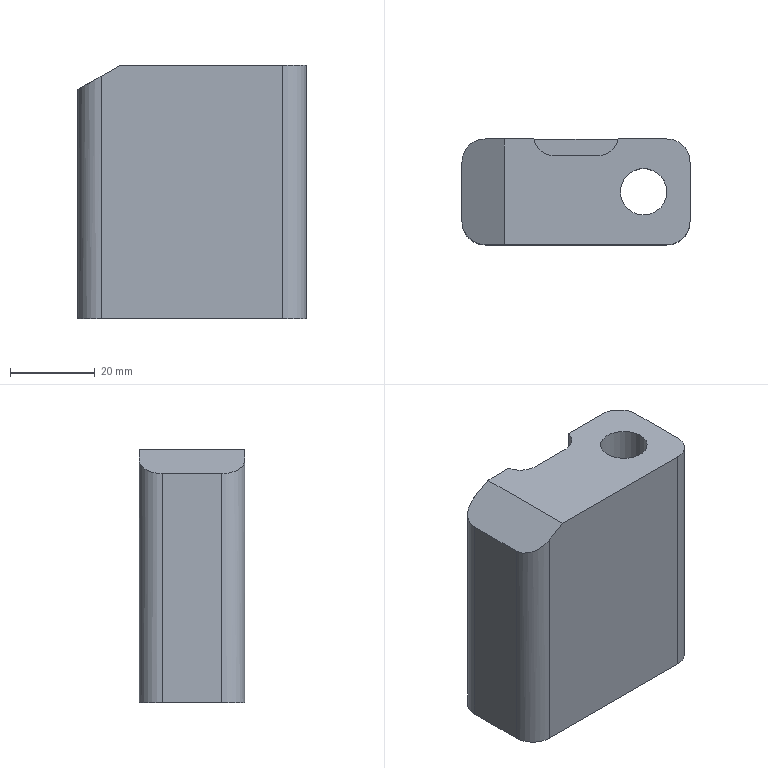Part | NX | features 1605338300 2 | 1 solid | 20 faces | box 54 x 25 x 60 mm | volume 60938 mm3 | plane 11 | cylinder 9 | commonest cylinder face diameters 11 x5 10 x2 17 x2
STEP:
#1=CARTESIAN_POINT('',(149.5,0.000000002,-61.5));
#2=VERTEX_POINT('',#1);
#3=CARTESIAN_POINT('',(158.,0.000000002,-61.5));
#4=DIRECTION('',(0.,0.,-1.));
#5=DIRECTION('',(-1.,0.,0.));
#6=AXIS2_PLACEMENT_3D('',#3,#4,#5);
#7=CIRCLE('',#6,8.5);
#8=EDGE_CURVE('',#2,#2,#7,.F.);
#9=ORIENTED_EDGE('',*,*,#8,.T.);
#10=EDGE_LOOP('',(#9));
#11=FACE_BOUND('',#10,.T.);
#12=CARTESIAN_POINT('',(147.,-7.,-61.5));
#13=VERTEX_POINT('',#12);
#14=CARTESIAN_POINT('',(147.,7.,-61.5));
#15=VERTEX_POINT('',#14);
#16=CARTESIAN_POINT('',(147.,-5.,-61.5));
#17=DIRECTION('',(0.,1.,0.));
#18=VECTOR('',#17,1000.);
#19=LINE('',#16,#18);
#20=EDGE_CURVE('',#13,#15,#19,.T.);
#21=ORIENTED_EDGE('',*,*,#20,.T.);
#22=CARTESIAN_POINT('',(152.5,12.5,-61.5));
#23=VERTEX_POINT('',#22);
#24=CARTESIAN_POINT('',(152.5,7.,-61.5));
#25=DIRECTION('',(0.,0.,-1.));
#26=DIRECTION('',(-1.,0.,0.));
#27=AXIS2_PLACEMENT_3D('',#24,#25,#26);
#28=CIRCLE('',#27,5.5);
#29=EDGE_CURVE('',#23,#15,#28,.F.);
#30=ORIENTED_EDGE('',*,*,#29,.F.);
#31=CARTESIAN_POINT('',(195.5,12.5,-61.5));
#32=VERTEX_POINT('',#31);
#33=CARTESIAN_POINT('',(159.,12.5,-61.5));
#34=DIRECTION('',(1.,0.,0.));
#35=VECTOR('',#34,1000.);
#36=LINE('',#33,#35);
#37=EDGE_CURVE('',#23,#32,#36,.T.);
#38=ORIENTED_EDGE('',*,*,#37,.T.);
#39=CARTESIAN_POINT('',(201.,7.,-61.5));
#40=VERTEX_POINT('',#39);
#41=CARTESIAN_POINT('',(195.5,7.,-61.5));
#42=DIRECTION('',(0.,0.,-1.));
#43=DIRECTION('',(-1.,0.,0.));
#44=AXIS2_PLACEMENT_3D('',#41,#42,#43);
#45=CIRCLE('',#44,5.5);
#46=EDGE_CURVE('',#40,#32,#45,.F.);
#47=ORIENTED_EDGE('',*,*,#46,.F.);
#48=CARTESIAN_POINT('',(201.,-7.,-61.5));
#49=VERTEX_POINT('',#48);
#50=CARTESIAN_POINT('',(201.,-5.,-61.5));
#51=DIRECTION('',(0.,-1.,0.));
#52=VECTOR('',#51,1000.);
#53=LINE('',#50,#52);
#54=EDGE_CURVE('',#40,#49,#53,.T.);
#55=ORIENTED_EDGE('',*,*,#54,.T.);
#56=CARTESIAN_POINT('',(195.5,-12.5,-61.5));
#57=VERTEX_POINT('',#56);
#58=CARTESIAN_POINT('',(195.5,-7.,-61.5));
#59=DIRECTION('',(0.,0.,-1.));
#60=DIRECTION('',(-1.,0.,0.));
#61=AXIS2_PLACEMENT_3D('',#58,#59,#60);
#62=CIRCLE('',#61,5.5);
#63=EDGE_CURVE('',#57,#49,#62,.F.);
#64=ORIENTED_EDGE('',*,*,#63,.F.);
#65=CARTESIAN_POINT('',(152.5,-12.5,-61.5));
#66=VERTEX_POINT('',#65);
#67=CARTESIAN_POINT('',(159.,-12.5,-61.5));
#68=DIRECTION('',(-1.,0.,0.));
#69=VECTOR('',#68,1000.);
#70=LINE('',#67,#69);
#71=EDGE_CURVE('',#57,#66,#70,.T.);
#72=ORIENTED_EDGE('',*,*,#71,.T.);
#73=CARTESIAN_POINT('',(152.5,-7.,-61.5));
#74=DIRECTION('',(0.,0.,-1.));
#75=DIRECTION('',(-1.,0.,0.));
#76=AXIS2_PLACEMENT_3D('',#73,#74,#75);
#77=CIRCLE('',#76,5.5);
#78=EDGE_CURVE('',#13,#66,#77,.F.);
#79=ORIENTED_EDGE('',*,*,#78,.F.);
#80=EDGE_LOOP('',(#21,#30,#38,#47,#55,#64,#72,#79));
#81=FACE_BOUND('',#80,.T.);
#82=CARTESIAN_POINT('',(181.5,0.000000002,-61.5));
#83=VERTEX_POINT('',#82);
#84=CARTESIAN_POINT('',(190.,0.000000002,-61.5));
#85=DIRECTION('',(0.,0.,-1.));
#86=DIRECTION('',(-1.,0.,0.));
#87=AXIS2_PLACEMENT_3D('',#84,#85,#86);
#88=CIRCLE('',#87,8.5);
#89=EDGE_CURVE('',#83,#83,#88,.F.);
#90=ORIENTED_EDGE('',*,*,#89,.T.);
#91=EDGE_LOOP('',(#90));
#92=FACE_BOUND('',#91,.T.);
#93=CARTESIAN_POINT('',(159.,-5.,-61.5));
#94=DIRECTION('',(0.,0.,-1.));
#95=DIRECTION('',(-1.,0.,0.));
#96=AXIS2_PLACEMENT_3D('',#93,#94,#95);
#97=PLANE('',#96);
#98=ADVANCED_FACE('',(#11,#81,#92),#97,.T.);
#99=CARTESIAN_POINT('',(181.5,0.000000002,-34.5));
#100=VERTEX_POINT('',#99);
#101=CARTESIAN_POINT('',(190.,0.000000002,-34.5));
#102=DIRECTION('',(0.,0.,-1.));
#103=DIRECTION('',(-1.,0.,0.));
#104=AXIS2_PLACEMENT_3D('',#101,#102,#103);
#105=CIRCLE('',#104,8.5);
#106=EDGE_CURVE('',#100,#100,#105,.T.);
#107=ORIENTED_EDGE('',*,*,#106,.F.);
#108=EDGE_LOOP('',(#107));
#109=FACE_BOUND('',#108,.T.);
#110=ORIENTED_EDGE('',*,*,#89,.F.);
#111=EDGE_LOOP('',(#110));
#112=FACE_BOUND('',#111,.T.);
#113=CARTESIAN_POINT('',(190.,0.000000002,-34.5));
#114=DIRECTION('',(0.,0.,-1.));
#115=DIRECTION('',(-1.,0.,0.));
#116=AXIS2_PLACEMENT_3D('',#113,#114,#115);
#117=CYLINDRICAL_SURFACE('',#116,8.5);
#118=ADVANCED_FACE('',(#109,#112),#117,.F.);
#119=CARTESIAN_POINT('',(184.5,0.,-34.5));
#120=VERTEX_POINT('',#119);
#121=CARTESIAN_POINT('',(190.,0.,-34.5));
#122=DIRECTION('',(0.,0.,-1.));
#123=DIRECTION('',(-1.,0.,0.));
#124=AXIS2_PLACEMENT_3D('',#121,#122,#123);
#125=CIRCLE('',#124,5.5);
#126=EDGE_CURVE('',#120,#120,#125,.T.);
#127=ORIENTED_EDGE('',*,*,#126,.T.);
#128=EDGE_LOOP('',(#127));
#129=FACE_BOUND('',#128,.T.);
#130=CARTESIAN_POINT('',(195.5,0.,-1.5));
#131=VERTEX_POINT('',#130);
#132=CARTESIAN_POINT('',(190.,0.,-1.5));
#133=DIRECTION('',(0.,0.,1.));
#134=DIRECTION('',(1.,0.,0.));
#135=AXIS2_PLACEMENT_3D('',#132,#133,#134);
#136=CIRCLE('',#135,5.5);
#137=EDGE_CURVE('',#131,#131,#136,.F.);
#138=ORIENTED_EDGE('',*,*,#137,.F.);
#139=EDGE_LOOP('',(#138));
#140=FACE_BOUND('',#139,.T.);
#141=CARTESIAN_POINT('',(190.,0.,20.5));
#142=DIRECTION('',(0.,0.,-1.));
#143=DIRECTION('',(-1.,0.,0.));
#144=AXIS2_PLACEMENT_3D('',#141,#142,#143);
#145=CYLINDRICAL_SURFACE('',#144,5.5);
#146=ADVANCED_FACE('',(#129,#140),#145,.F.);
#147=ORIENTED_EDGE('',*,*,#137,.T.);
#148=EDGE_LOOP('',(#147));
#149=FACE_BOUND('',#148,.T.);
#150=CARTESIAN_POINT('',(168.899,8.5,-1.5));
#151=VERTEX_POINT('',#150);
#152=CARTESIAN_POINT('',(179.101,8.5,-1.5));
#153=VERTEX_POINT('',#152);
#154=CARTESIAN_POINT('',(170.,8.5,-1.5));
#155=DIRECTION('',(1.,0.,0.));
#156=VECTOR('',#155,1000.);
#157=LINE('',#154,#156);
#158=EDGE_CURVE('',#151,#153,#157,.T.);
#159=ORIENTED_EDGE('',*,*,#158,.F.);
#160=CARTESIAN_POINT('',(164.,12.5,-1.5));
#161=VERTEX_POINT('',#160);
#162=CARTESIAN_POINT('',(168.899,13.5,-1.5));
#163=DIRECTION('',(0.,0.,-1.));
#164=DIRECTION('',(1.,0.,0.));
#165=AXIS2_PLACEMENT_3D('',#162,#163,#164);
#166=CIRCLE('',#165,5.);
#167=EDGE_CURVE('',#161,#151,#166,.F.);
#168=ORIENTED_EDGE('',*,*,#167,.F.);
#169=CARTESIAN_POINT('',(157.,12.5,-1.5));
#170=VERTEX_POINT('',#169);
#171=CARTESIAN_POINT('',(159.,12.5,-1.5));
#172=DIRECTION('',(-1.,0.,0.));
#173=VECTOR('',#172,1000.);
#174=LINE('',#171,#173);
#175=EDGE_CURVE('',#161,#170,#174,.T.);
#176=ORIENTED_EDGE('',*,*,#175,.T.);
#177=CARTESIAN_POINT('',(157.,-12.5,-1.5));
#178=VERTEX_POINT('',#177);
#179=CARTESIAN_POINT('',(157.,-5.,-1.5));
#180=DIRECTION('',(0.,1.,0.));
#181=VECTOR('',#180,1000.);
#182=LINE('',#179,#181);
#183=EDGE_CURVE('',#178,#170,#182,.T.);
#184=ORIENTED_EDGE('',*,*,#183,.F.);
#185=CARTESIAN_POINT('',(195.5,-12.5,-1.5));
#186=VERTEX_POINT('',#185);
#187=CARTESIAN_POINT('',(159.,-12.5,-1.5));
#188=DIRECTION('',(1.,0.,0.));
#189=VECTOR('',#188,1000.);
#190=LINE('',#187,#189);
#191=EDGE_CURVE('',#178,#186,#190,.T.);
#192=ORIENTED_EDGE('',*,*,#191,.T.);
#193=CARTESIAN_POINT('',(201.,-7.,-1.5));
#194=VERTEX_POINT('',#193);
#195=CARTESIAN_POINT('',(195.5,-7.,-1.5));
#196=DIRECTION('',(0.,0.,1.));
#197=DIRECTION('',(1.,0.,0.));
#198=AXIS2_PLACEMENT_3D('',#195,#196,#197);
#199=CIRCLE('',#198,5.5);
#200=EDGE_CURVE('',#194,#186,#199,.F.);
#201=ORIENTED_EDGE('',*,*,#200,.F.);
#202=CARTESIAN_POINT('',(201.,7.,-1.5));
#203=VERTEX_POINT('',#202);
#204=CARTESIAN_POINT('',(201.,-5.,-1.5));
#205=DIRECTION('',(0.,1.,0.));
#206=VECTOR('',#205,1000.);
#207=LINE('',#204,#206);
#208=EDGE_CURVE('',#194,#203,#207,.T.);
#209=ORIENTED_EDGE('',*,*,#208,.T.);
#210=CARTESIAN_POINT('',(195.5,12.5,-1.5));
#211=VERTEX_POINT('',#210);
#212=CARTESIAN_POINT('',(195.5,7.,-1.5));
#213=DIRECTION('',(0.,0.,1.));
#214=DIRECTION('',(1.,0.,0.));
#215=AXIS2_PLACEMENT_3D('',#212,#213,#214);
#216=CIRCLE('',#215,5.5);
#217=EDGE_CURVE('',#211,#203,#216,.F.);
#218=ORIENTED_EDGE('',*,*,#217,.F.);
#219=CARTESIAN_POINT('',(184.,12.5,-1.5));
#220=VERTEX_POINT('',#219);
#221=CARTESIAN_POINT('',(159.,12.5,-1.5));
#222=DIRECTION('',(-1.,0.,0.));
#223=VECTOR('',#222,1000.);
#224=LINE('',#221,#223);
#225=EDGE_CURVE('',#211,#220,#224,.T.);
#226=ORIENTED_EDGE('',*,*,#225,.T.);
#227=CARTESIAN_POINT('',(179.101,13.5,-1.5));
#228=DIRECTION('',(0.,0.,-1.));
#229=DIRECTION('',(1.,0.,0.));
#230=AXIS2_PLACEMENT_3D('',#227,#228,#229);
#231=CIRCLE('',#230,5.);
#232=EDGE_CURVE('',#153,#220,#231,.F.);
#233=ORIENTED_EDGE('',*,*,#232,.F.);
#234=EDGE_LOOP('',(#159,#168,#176,#184,#192,#201,#209,#218,#226,#233));
#235=FACE_BOUND('',#234,.T.);
#236=CARTESIAN_POINT('',(159.,-5.,-1.5));
#237=DIRECTION('',(0.,0.,1.));
#238=DIRECTION('',(1.,0.,0.));
#239=AXIS2_PLACEMENT_3D('',#236,#237,#238);
#240=PLANE('',#239);
#241=ADVANCED_FACE('',(#149,#235),#240,.T.);
#242=ORIENTED_EDGE('',*,*,#71,.F.);
#243=CARTESIAN_POINT('',(195.5,-12.5,-1.5));
#244=DIRECTION('',(0.,0.,-1.));
#245=VECTOR('',#244,1000.);
#246=LINE('',#243,#245);
#247=EDGE_CURVE('',#186,#57,#246,.T.);
#248=ORIENTED_EDGE('',*,*,#247,.F.);
#249=ORIENTED_EDGE('',*,*,#191,.F.);
#250=CARTESIAN_POINT('',(152.5,-12.5,-4.098));
#251=VERTEX_POINT('',#250);
#252=CARTESIAN_POINT('',(157.,-12.5,-1.5));
#253=DIRECTION('',(-0.866,0.,-0.5));
#254=VECTOR('',#253,1000.);
#255=LINE('',#252,#254);
#256=EDGE_CURVE('',#251,#178,#255,.F.);
#257=ORIENTED_EDGE('',*,*,#256,.F.);
#258=CARTESIAN_POINT('',(152.5,-12.5,-1.5));
#259=DIRECTION('',(0.,0.,-1.));
#260=VECTOR('',#259,1000.);
#261=LINE('',#258,#260);
#262=EDGE_CURVE('',#66,#251,#261,.F.);
#263=ORIENTED_EDGE('',*,*,#262,.F.);
#264=EDGE_LOOP('',(#242,#248,#249,#257,#263));
#265=FACE_BOUND('',#264,.T.);
#266=CARTESIAN_POINT('',(159.,-12.5,-1.5));
#267=DIRECTION('',(0.,-1.,0.));
#268=DIRECTION('',(0.,0.,1.));
#269=AXIS2_PLACEMENT_3D('',#266,#267,#268);
#270=PLANE('',#269);
#271=ADVANCED_FACE('',(#265),#270,.T.);
#272=CARTESIAN_POINT('',(147.,7.,-7.274));
#273=VERTEX_POINT('',#272);
#274=CARTESIAN_POINT('',(147.,-7.,-7.274));
#275=VERTEX_POINT('',#274);
#276=CARTESIAN_POINT('',(147.,-5.,-7.274));
#277=DIRECTION('',(0.,-1.,0.));
#278=VECTOR('',#277,1000.);
#279=LINE('',#276,#278);
#280=EDGE_CURVE('',#273,#275,#279,.T.);
#281=ORIENTED_EDGE('',*,*,#280,.F.);
#282=CARTESIAN_POINT('',(147.,7.,-1.5));
#283=DIRECTION('',(0.,0.,-1.));
#284=VECTOR('',#283,1000.);
#285=LINE('',#282,#284);
#286=EDGE_CURVE('',#15,#273,#285,.F.);
#287=ORIENTED_EDGE('',*,*,#286,.F.);
#288=ORIENTED_EDGE('',*,*,#20,.F.);
#289=CARTESIAN_POINT('',(147.,-7.,-1.5));
#290=DIRECTION('',(0.,0.,-1.));
#291=VECTOR('',#290,1000.);
#292=LINE('',#289,#291);
#293=EDGE_CURVE('',#275,#13,#292,.T.);
#294=ORIENTED_EDGE('',*,*,#293,.F.);
#295=EDGE_LOOP('',(#281,#287,#288,#294));
#296=FACE_BOUND('',#295,.T.);
#297=CARTESIAN_POINT('',(147.,-5.,-1.5));
#298=DIRECTION('',(-1.,0.,0.));
#299=DIRECTION('',(0.,0.,1.));
#300=AXIS2_PLACEMENT_3D('',#297,#298,#299);
#301=PLANE('',#300);
#302=ADVANCED_FACE('',(#296),#301,.T.);
#303=CARTESIAN_POINT('',(164.,12.5,-36.5));
#304=VERTEX_POINT('',#303);
#305=CARTESIAN_POINT('',(164.,12.5,-1.5));
#306=DIRECTION('',(0.,0.,-1.));
#307=VECTOR('',#306,1000.);
#308=LINE('',#305,#307);
#309=EDGE_CURVE('',#161,#304,#308,.T.);
#310=ORIENTED_EDGE('',*,*,#309,.T.);
#311=CARTESIAN_POINT('',(184.,12.5,-36.5));
#312=VERTEX_POINT('',#311);
#313=CARTESIAN_POINT('',(159.,12.5,-36.5));
#314=DIRECTION('',(1.,0.,0.));
#315=VECTOR('',#314,1000.);
#316=LINE('',#313,#315);
#317=EDGE_CURVE('',#304,#312,#316,.T.);
#318=ORIENTED_EDGE('',*,*,#317,.T.);
#319=CARTESIAN_POINT('',(184.,12.5,-1.5));
#320=DIRECTION('',(0.,0.,1.));
#321=VECTOR('',#320,1000.);
#322=LINE('',#319,#321);
#323=EDGE_CURVE('',#312,#220,#322,.T.);
#324=ORIENTED_EDGE('',*,*,#323,.T.);
#325=ORIENTED_EDGE('',*,*,#225,.F.);
#326=CARTESIAN_POINT('',(195.5,12.5,-1.5));
#327=DIRECTION('',(0.,0.,-1.));
#328=VECTOR('',#327,1000.);
#329=LINE('',#326,#328);
#330=EDGE_CURVE('',#32,#211,#329,.F.);
#331=ORIENTED_EDGE('',*,*,#330,.F.);
#332=ORIENTED_EDGE('',*,*,#37,.F.);
#333=CARTESIAN_POINT('',(152.5,12.5,-4.098));
#334=VERTEX_POINT('',#333);
#335=CARTESIAN_POINT('',(152.5,12.5,-1.5));
#336=DIRECTION('',(0.,0.,-1.));
#337=VECTOR('',#336,1000.);
#338=LINE('',#335,#337);
#339=EDGE_CURVE('',#334,#23,#338,.T.);
#340=ORIENTED_EDGE('',*,*,#339,.F.);
#341=CARTESIAN_POINT('',(157.,12.5,-1.5));
#342=DIRECTION('',(0.866,0.,0.5));
#343=VECTOR('',#342,1000.);
#344=LINE('',#341,#343);
#345=EDGE_CURVE('',#170,#334,#344,.F.);
#346=ORIENTED_EDGE('',*,*,#345,.F.);
#347=ORIENTED_EDGE('',*,*,#175,.F.);
#348=EDGE_LOOP('',(#310,#318,#324,#325,#331,#332,#340,#346,#347));
#349=FACE_BOUND('',#348,.T.);
#350=CARTESIAN_POINT('',(159.,12.5,-1.5));
#351=DIRECTION('',(0.,1.,0.));
#352=DIRECTION('',(0.,0.,-1.));
#353=AXIS2_PLACEMENT_3D('',#350,#351,#352);
#354=PLANE('',#353);
#355=ADVANCED_FACE('',(#349),#354,.T.);
#356=ORIENTED_EDGE('',*,*,#54,.F.);
#357=CARTESIAN_POINT('',(201.,7.,-1.5));
#358=DIRECTION('',(0.,0.,-1.));
#359=VECTOR('',#358,1000.);
#360=LINE('',#357,#359);
#361=EDGE_CURVE('',#203,#40,#360,.T.);
#362=ORIENTED_EDGE('',*,*,#361,.F.);
#363=ORIENTED_EDGE('',*,*,#208,.F.);
#364=CARTESIAN_POINT('',(201.,-7.,-1.5));
#365=DIRECTION('',(0.,0.,-1.));
#366=VECTOR('',#365,1000.);
#367=LINE('',#364,#366);
#368=EDGE_CURVE('',#49,#194,#367,.F.);
#369=ORIENTED_EDGE('',*,*,#368,.F.);
#370=EDGE_LOOP('',(#356,#362,#363,#369));
#371=FACE_BOUND('',#370,.T.);
#372=CARTESIAN_POINT('',(201.,-5.,-1.5));
#373=DIRECTION('',(1.,0.,0.));
#374=DIRECTION('',(0.,0.,-1.));
#375=AXIS2_PLACEMENT_3D('',#372,#373,#374);
#376=PLANE('',#375);
#377=ADVANCED_FACE('',(#371),#376,.T.);
#378=ORIENTED_EDGE('',*,*,#256,.T.);
#379=ORIENTED_EDGE('',*,*,#183,.T.);
#380=ORIENTED_EDGE('',*,*,#345,.T.);
#381=CARTESIAN_POINT('',(152.5,7.,-4.098));
#382=DIRECTION('',(0.5,0.,-0.866));
#383=DIRECTION('',(0.866,0.,0.5));
#384=AXIS2_PLACEMENT_3D('',#381,#382,#383);
#385=ELLIPSE('',#384,6.351,5.5);
#386=EDGE_CURVE('',#273,#334,#385,.T.);
#387=ORIENTED_EDGE('',*,*,#386,.F.);
#388=ORIENTED_EDGE('',*,*,#280,.T.);
#389=CARTESIAN_POINT('',(152.5,-7.,-4.098));
#390=DIRECTION('',(0.5,0.,-0.866));
#391=DIRECTION('',(0.866,0.,0.5));
#392=AXIS2_PLACEMENT_3D('',#389,#390,#391);
#393=ELLIPSE('',#392,6.351,5.5);
#394=EDGE_CURVE('',#251,#275,#393,.T.);
#395=ORIENTED_EDGE('',*,*,#394,.F.);
#396=EDGE_LOOP('',(#378,#379,#380,#387,#388,#395));
#397=FACE_BOUND('',#396,.T.);
#398=CARTESIAN_POINT('',(147.,-5.,-7.274));
#399=DIRECTION('',(0.5,0.,-0.866));
#400=DIRECTION('',(-0.866,0.,-0.5));
#401=AXIS2_PLACEMENT_3D('',#398,#399,#400);
#402=PLANE('',#401);
#403=ADVANCED_FACE('',(#397),#402,.F.);
#404=ORIENTED_EDGE('',*,*,#217,.T.);
#405=ORIENTED_EDGE('',*,*,#361,.T.);
#406=ORIENTED_EDGE('',*,*,#46,.T.);
#407=ORIENTED_EDGE('',*,*,#330,.T.);
#408=EDGE_LOOP('',(#404,#405,#406,#407));
#409=FACE_BOUND('',#408,.T.);
#410=CARTESIAN_POINT('',(195.5,7.,-1.5));
#411=DIRECTION('',(0.,0.,1.));
#412=DIRECTION('',(1.,0.,0.));
#413=AXIS2_PLACEMENT_3D('',#410,#411,#412);
#414=CYLINDRICAL_SURFACE('',#413,5.5);
#415=ADVANCED_FACE('',(#409),#414,.T.);
#416=ORIENTED_EDGE('',*,*,#200,.T.);
#417=ORIENTED_EDGE('',*,*,#247,.T.);
#418=ORIENTED_EDGE('',*,*,#63,.T.);
#419=ORIENTED_EDGE('',*,*,#368,.T.);
#420=EDGE_LOOP('',(#416,#417,#418,#419));
#421=FACE_BOUND('',#420,.T.);
#422=CARTESIAN_POINT('',(195.5,-7.,-1.5));
#423=DIRECTION('',(0.,0.,1.));
#424=DIRECTION('',(1.,0.,0.));
#425=AXIS2_PLACEMENT_3D('',#422,#423,#424);
#426=CYLINDRICAL_SURFACE('',#425,5.5);
#427=ADVANCED_FACE('',(#421),#426,.T.);
#428=ORIENTED_EDGE('',*,*,#386,.T.);
#429=ORIENTED_EDGE('',*,*,#339,.T.);
#430=ORIENTED_EDGE('',*,*,#29,.T.);
#431=ORIENTED_EDGE('',*,*,#286,.T.);
#432=EDGE_LOOP('',(#428,#429,#430,#431));
#433=FACE_BOUND('',#432,.T.);
#434=CARTESIAN_POINT('',(152.5,7.,-1.5));
#435=DIRECTION('',(0.,0.,1.));
#436=DIRECTION('',(1.,0.,0.));
#437=AXIS2_PLACEMENT_3D('',#434,#435,#436);
#438=CYLINDRICAL_SURFACE('',#437,5.5);
#439=ADVANCED_FACE('',(#433),#438,.T.);
#440=ORIENTED_EDGE('',*,*,#394,.T.);
#441=ORIENTED_EDGE('',*,*,#293,.T.);
#442=ORIENTED_EDGE('',*,*,#78,.T.);
#443=ORIENTED_EDGE('',*,*,#262,.T.);
#444=EDGE_LOOP('',(#440,#441,#442,#443));
#445=FACE_BOUND('',#444,.T.);
#446=CARTESIAN_POINT('',(152.5,-7.,-1.5));
#447=DIRECTION('',(0.,0.,1.));
#448=DIRECTION('',(1.,0.,0.));
#449=AXIS2_PLACEMENT_3D('',#446,#447,#448);
#450=CYLINDRICAL_SURFACE('',#449,5.5);
#451=ADVANCED_FACE('',(#445),#450,.T.);
#452=CARTESIAN_POINT('',(168.899,8.5,-36.5));
#453=VERTEX_POINT('',#452);
#454=CARTESIAN_POINT('',(179.101,8.5,-36.5));
#455=VERTEX_POINT('',#454);
#456=CARTESIAN_POINT('',(166.,8.5,-36.5));
#457=DIRECTION('',(1.,0.,0.));
#458=VECTOR('',#457,1000.);
#459=LINE('',#456,#458);
#460=EDGE_CURVE('',#453,#455,#459,.T.);
#461=ORIENTED_EDGE('',*,*,#460,.F.);
#462=CARTESIAN_POINT('',(168.899,8.5,-16.5));
#463=DIRECTION('',(0.,0.,1.));
#464=VECTOR('',#463,1000.);
#465=LINE('',#462,#464);
#466=EDGE_CURVE('',#151,#453,#465,.F.);
#467=ORIENTED_EDGE('',*,*,#466,.F.);
#468=ORIENTED_EDGE('',*,*,#158,.T.);
#469=CARTESIAN_POINT('',(179.101,8.5,-16.5));
#470=DIRECTION('',(0.,0.,-1.));
#471=VECTOR('',#470,1000.);
#472=LINE('',#469,#471);
#473=EDGE_CURVE('',#455,#153,#472,.F.);
#474=ORIENTED_EDGE('',*,*,#473,.F.);
#475=EDGE_LOOP('',(#461,#467,#468,#474));
#476=FACE_BOUND('',#475,.T.);
#477=CARTESIAN_POINT('',(170.,8.5,-16.5));
#478=DIRECTION('',(0.,-1.,0.));
#479=DIRECTION('',(0.,0.,1.));
#480=AXIS2_PLACEMENT_3D('',#477,#478,#479);
#481=PLANE('',#480);
#482=ADVANCED_FACE('',(#476),#481,.F.);
#483=ORIENTED_EDGE('',*,*,#317,.F.);
#484=CARTESIAN_POINT('',(168.899,13.5,-36.5));
#485=DIRECTION('',(0.,0.,1.));
#486=DIRECTION('',(1.,0.,0.));
#487=AXIS2_PLACEMENT_3D('',#484,#485,#486);
#488=CIRCLE('',#487,5.);
#489=EDGE_CURVE('',#453,#304,#488,.F.);
#490=ORIENTED_EDGE('',*,*,#489,.F.);
#491=ORIENTED_EDGE('',*,*,#460,.T.);
#492=CARTESIAN_POINT('',(179.101,13.5,-36.5));
#493=DIRECTION('',(0.,0.,1.));
#494=DIRECTION('',(1.,0.,0.));
#495=AXIS2_PLACEMENT_3D('',#492,#493,#494);
#496=CIRCLE('',#495,5.);
#497=EDGE_CURVE('',#312,#455,#496,.F.);
#498=ORIENTED_EDGE('',*,*,#497,.F.);
#499=EDGE_LOOP('',(#483,#490,#491,#498));
#500=FACE_BOUND('',#499,.T.);
#501=CARTESIAN_POINT('',(166.,12.5,-36.5));
#502=DIRECTION('',(0.,0.,1.));
#503=DIRECTION('',(1.,0.,0.));
#504=AXIS2_PLACEMENT_3D('',#501,#502,#503);
#505=PLANE('',#504);
#506=ADVANCED_FACE('',(#500),#505,.T.);
#507=ORIENTED_EDGE('',*,*,#489,.T.);
#508=ORIENTED_EDGE('',*,*,#309,.F.);
#509=ORIENTED_EDGE('',*,*,#167,.T.);
#510=ORIENTED_EDGE('',*,*,#466,.T.);
#511=EDGE_LOOP('',(#507,#508,#509,#510));
#512=FACE_BOUND('',#511,.T.);
#513=CARTESIAN_POINT('',(168.899,13.5,-16.5));
#514=DIRECTION('',(0.,0.,1.));
#515=DIRECTION('',(1.,0.,0.));
#516=AXIS2_PLACEMENT_3D('',#513,#514,#515);
#517=CYLINDRICAL_SURFACE('',#516,5.);
#518=ADVANCED_FACE('',(#512),#517,.F.);
#519=ORIENTED_EDGE('',*,*,#497,.T.);
#520=ORIENTED_EDGE('',*,*,#473,.T.);
#521=ORIENTED_EDGE('',*,*,#232,.T.);
#522=ORIENTED_EDGE('',*,*,#323,.F.);
#523=EDGE_LOOP('',(#519,#520,#521,#522));
#524=FACE_BOUND('',#523,.T.);
#525=CARTESIAN_POINT('',(179.101,13.5,-16.5));
#526=DIRECTION('',(0.,0.,-1.));
#527=DIRECTION('',(-1.,0.,0.));
#528=AXIS2_PLACEMENT_3D('',#525,#526,#527);
#529=CYLINDRICAL_SURFACE('',#528,5.);
#530=ADVANCED_FACE('',(#524),#529,.F.);
#531=ORIENTED_EDGE('',*,*,#106,.T.);
#532=EDGE_LOOP('',(#531));
#533=FACE_BOUND('',#532,.T.);
#534=ORIENTED_EDGE('',*,*,#126,.F.);
#535=EDGE_LOOP('',(#534));
#536=FACE_BOUND('',#535,.T.);
#537=CARTESIAN_POINT('',(140.,-64.5,-34.5));
#538=DIRECTION('',(0.,0.,-1.));
#539=DIRECTION('',(-1.,0.,0.));
#540=AXIS2_PLACEMENT_3D('',#537,#538,#539);
#541=PLANE('',#540);
#542=ADVANCED_FACE('',(#533,#536),#541,.T.);
#543=ORIENTED_EDGE('',*,*,#8,.F.);
#544=EDGE_LOOP('',(#543));
#545=FACE_BOUND('',#544,.T.);
#546=CARTESIAN_POINT('',(149.5,0.000000002,-34.5));
#547=VERTEX_POINT('',#546);
#548=CARTESIAN_POINT('',(158.,0.000000002,-34.5));
#549=DIRECTION('',(0.,0.,-1.));
#550=DIRECTION('',(-1.,0.,0.));
#551=AXIS2_PLACEMENT_3D('',#548,#549,#550);
#552=CIRCLE('',#551,8.5);
#553=EDGE_CURVE('',#547,#547,#552,.T.);
#554=ORIENTED_EDGE('',*,*,#553,.F.);
#555=EDGE_LOOP('',(#554));
#556=FACE_BOUND('',#555,.T.);
#557=CARTESIAN_POINT('',(158.,0.000000002,-34.5));
#558=DIRECTION('',(0.,0.,-1.));
#559=DIRECTION('',(-1.,0.,0.));
#560=AXIS2_PLACEMENT_3D('',#557,#558,#559);
#561=CYLINDRICAL_SURFACE('',#560,8.5);
#562=ADVANCED_FACE('',(#545,#556),#561,.F.);
#563=ORIENTED_EDGE('',*,*,#553,.T.);
#564=EDGE_LOOP('',(#563));
#565=FACE_BOUND('',#564,.T.);
#566=CARTESIAN_POINT('',(108.,-64.5,-34.5));
#567=DIRECTION('',(0.,0.,-1.));
#568=DIRECTION('',(-1.,0.,0.));
#569=AXIS2_PLACEMENT_3D('',#566,#567,#568);
#570=PLANE('',#569);
#571=ADVANCED_FACE('',(#565),#570,.T.);
#572=CLOSED_SHELL('',(#98,#118,#146,#241,#271,#302,#355,#377,#403,#415,#427,#439,#451,#482,#506,#518,#530,#542,#562,#571));
#573=MANIFOLD_SOLID_BREP('',#572);
#574=(LENGTH_UNIT()NAMED_UNIT(*)SI_UNIT(.MILLI.,.METRE.));
#575=UNCERTAINTY_MEASURE_WITH_UNIT(LENGTH_MEASURE(0.00001),#574,'','');
#576=(NAMED_UNIT(*)PLANE_ANGLE_UNIT()SI_UNIT($,.RADIAN.));
#577=(NAMED_UNIT(*)SI_UNIT($,.STERADIAN.)SOLID_ANGLE_UNIT());
#578=(GEOMETRIC_REPRESENTATION_CONTEXT(3)GLOBAL_UNCERTAINTY_ASSIGNED_CONTEXT((#575))GLOBAL_UNIT_ASSIGNED_CONTEXT((#574,#576,#577))REPRESENTATION_CONTEXT('',''));
#579=ADVANCED_BREP_SHAPE_REPRESENTATION('',(#573),#578);